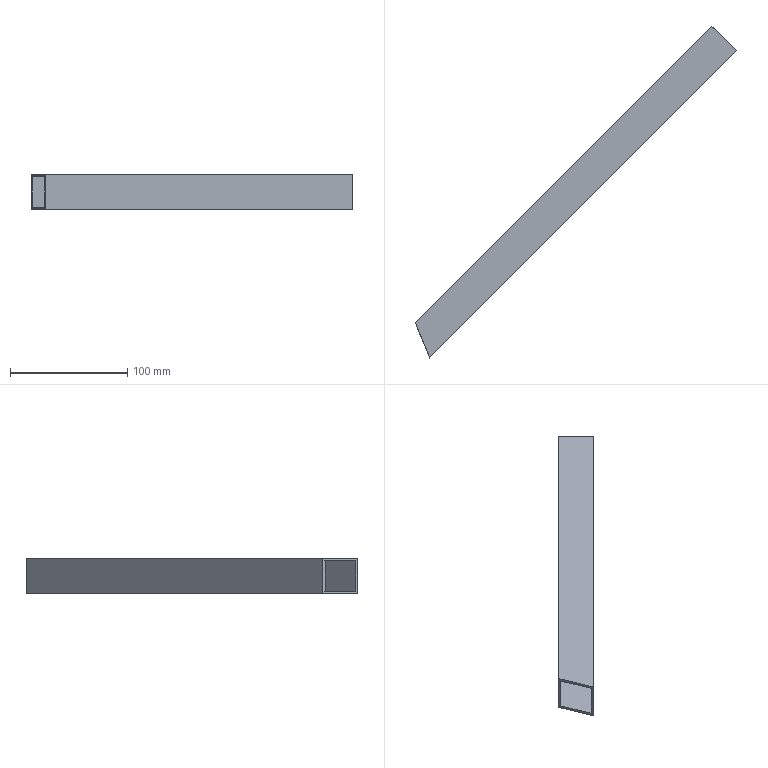Part | NX | features solid 2 | 1 solid | 10 faces | box 274.056 x 282.843 x 30 mm | volume 81488 mm3 | plane 10
STEP:
#1=CARTESIAN_POINT('',(696.63,501.63,-140.));
#2=VERTEX_POINT('',#1);
#3=CARTESIAN_POINT('',(675.416,522.843,-140.));
#4=VERTEX_POINT('',#3);
#5=CARTESIAN_POINT('',(696.63,501.63,-140.));
#6=DIRECTION('',(-0.7071,0.7071,0.));
#7=VECTOR('',#6,1000.);
#8=LINE('',#5,#7);
#9=EDGE_CURVE('',#2,#4,#8,.T.);
#10=ORIENTED_EDGE('',*,*,#9,.T.);
#11=CARTESIAN_POINT('',(675.416,522.843,-110.));
#12=VERTEX_POINT('',#11);
#13=CARTESIAN_POINT('',(675.416,522.843,-110.));
#14=DIRECTION('',(0.,0.,-1.));
#15=VECTOR('',#14,1000.);
#16=LINE('',#13,#15);
#17=EDGE_CURVE('',#12,#4,#16,.T.);
#18=ORIENTED_EDGE('',*,*,#17,.F.);
#19=CARTESIAN_POINT('',(696.63,501.63,-110.));
#20=VERTEX_POINT('',#19);
#21=CARTESIAN_POINT('',(696.63,501.63,-110.));
#22=DIRECTION('',(-0.7071,0.7071,0.));
#23=VECTOR('',#22,1000.);
#24=LINE('',#21,#23);
#25=EDGE_CURVE('',#20,#12,#24,.T.);
#26=ORIENTED_EDGE('',*,*,#25,.F.);
#27=CARTESIAN_POINT('',(696.63,501.63,-110.));
#28=DIRECTION('',(0.,0.,-1.));
#29=VECTOR('',#28,1000.);
#30=LINE('',#27,#29);
#31=EDGE_CURVE('',#20,#2,#30,.T.);
#32=ORIENTED_EDGE('',*,*,#31,.T.);
#33=EDGE_LOOP('',(#10,#18,#26,#32));
#34=FACE_BOUND('',#33,.T.);
#35=CARTESIAN_POINT('',(695.215,503.044,-112.));
#36=VERTEX_POINT('',#35);
#37=CARTESIAN_POINT('',(695.215,503.044,-138.));
#38=VERTEX_POINT('',#37);
#39=CARTESIAN_POINT('',(695.215,503.044,-110.));
#40=DIRECTION('',(0.,0.,-1.));
#41=VECTOR('',#40,1000.);
#42=LINE('',#39,#41);
#43=EDGE_CURVE('',#36,#38,#42,.T.);
#44=ORIENTED_EDGE('',*,*,#43,.F.);
#45=CARTESIAN_POINT('',(676.831,521.428,-112.));
#46=VERTEX_POINT('',#45);
#47=CARTESIAN_POINT('',(696.63,501.63,-112.));
#48=DIRECTION('',(-0.7071,0.7071,0.));
#49=VECTOR('',#48,1000.);
#50=LINE('',#47,#49);
#51=EDGE_CURVE('',#36,#46,#50,.T.);
#52=ORIENTED_EDGE('',*,*,#51,.T.);
#53=CARTESIAN_POINT('',(676.831,521.428,-138.));
#54=VERTEX_POINT('',#53);
#55=CARTESIAN_POINT('',(676.831,521.428,-110.));
#56=DIRECTION('',(0.,0.,-1.));
#57=VECTOR('',#56,1000.);
#58=LINE('',#55,#57);
#59=EDGE_CURVE('',#46,#54,#58,.T.);
#60=ORIENTED_EDGE('',*,*,#59,.T.);
#61=CARTESIAN_POINT('',(696.63,501.63,-138.));
#62=DIRECTION('',(-0.7071,0.7071,0.));
#63=VECTOR('',#62,1000.);
#64=LINE('',#61,#63);
#65=EDGE_CURVE('',#38,#54,#64,.T.);
#66=ORIENTED_EDGE('',*,*,#65,.F.);
#67=EDGE_LOOP('',(#44,#52,#60,#66));
#68=FACE_BOUND('',#67,.T.);
#69=CARTESIAN_POINT('',(696.63,501.63,-110.));
#70=DIRECTION('',(0.7071,0.7071,0.));
#71=DIRECTION('',(0.7071,-0.7071,0.));
#72=AXIS2_PLACEMENT_3D('',#69,#70,#71);
#73=PLANE('',#72);
#74=ADVANCED_FACE('',(#34,#68),#73,.T.);
#75=CARTESIAN_POINT('',(435.,240.,-140.));
#76=VERTEX_POINT('',#75);
#77=CARTESIAN_POINT('',(435.,240.,-140.));
#78=DIRECTION('',(0.7071,0.7071,0.));
#79=VECTOR('',#78,1000.);
#80=LINE('',#77,#79);
#81=EDGE_CURVE('',#76,#2,#80,.T.);
#82=ORIENTED_EDGE('',*,*,#81,.T.);
#83=ORIENTED_EDGE('',*,*,#31,.F.);
#84=CARTESIAN_POINT('',(435.,240.,-110.));
#85=VERTEX_POINT('',#84);
#86=CARTESIAN_POINT('',(435.,240.,-110.));
#87=DIRECTION('',(0.7071,0.7071,0.));
#88=VECTOR('',#87,1000.);
#89=LINE('',#86,#88);
#90=EDGE_CURVE('',#85,#20,#89,.T.);
#91=ORIENTED_EDGE('',*,*,#90,.F.);
#92=CARTESIAN_POINT('',(435.,240.,-110.));
#93=DIRECTION('',(0.,0.,-1.));
#94=VECTOR('',#93,1000.);
#95=LINE('',#92,#94);
#96=EDGE_CURVE('',#85,#76,#95,.T.);
#97=ORIENTED_EDGE('',*,*,#96,.T.);
#98=EDGE_LOOP('',(#82,#83,#91,#97));
#99=FACE_BOUND('',#98,.T.);
#100=CARTESIAN_POINT('',(435.,240.,-110.));
#101=DIRECTION('',(0.7071,-0.7071,0.));
#102=DIRECTION('',(-0.7071,-0.7071,0.));
#103=AXIS2_PLACEMENT_3D('',#100,#101,#102);
#104=PLANE('',#103);
#105=ADVANCED_FACE('',(#99),#104,.T.);
#106=CARTESIAN_POINT('',(422.574,270.,-110.));
#107=VERTEX_POINT('',#106);
#108=CARTESIAN_POINT('',(392.574,240.,-110.));
#109=DIRECTION('',(0.7071,0.7071,0.));
#110=VECTOR('',#109,1000.);
#111=LINE('',#108,#110);
#112=EDGE_CURVE('',#107,#12,#111,.T.);
#113=ORIENTED_EDGE('',*,*,#112,.T.);
#114=ORIENTED_EDGE('',*,*,#17,.T.);
#115=CARTESIAN_POINT('',(422.574,270.,-140.));
#116=VERTEX_POINT('',#115);
#117=CARTESIAN_POINT('',(392.574,240.,-140.));
#118=DIRECTION('',(0.7071,0.7071,0.));
#119=VECTOR('',#118,1000.);
#120=LINE('',#117,#119);
#121=EDGE_CURVE('',#116,#4,#120,.T.);
#122=ORIENTED_EDGE('',*,*,#121,.F.);
#123=CARTESIAN_POINT('',(422.574,270.,-110.));
#124=DIRECTION('',(0.,0.,-1.));
#125=VECTOR('',#124,1000.);
#126=LINE('',#123,#125);
#127=EDGE_CURVE('',#107,#116,#126,.T.);
#128=ORIENTED_EDGE('',*,*,#127,.F.);
#129=EDGE_LOOP('',(#113,#114,#122,#128));
#130=FACE_BOUND('',#129,.T.);
#131=CARTESIAN_POINT('',(392.574,240.,-110.));
#132=DIRECTION('',(0.7071,-0.7071,0.));
#133=DIRECTION('',(-0.7071,-0.7071,0.));
#134=AXIS2_PLACEMENT_3D('',#131,#132,#133);
#135=PLANE('',#134);
#136=ADVANCED_FACE('',(#130),#135,.F.);
#137=CARTESIAN_POINT('',(419.9,276.454,-110.));
#138=DIRECTION('',(0.3827,-0.9239,0.));
#139=VECTOR('',#138,1000.);
#140=LINE('',#137,#139);
#141=EDGE_CURVE('',#107,#85,#140,.T.);
#142=ORIENTED_EDGE('',*,*,#141,.T.);
#143=ORIENTED_EDGE('',*,*,#90,.T.);
#144=ORIENTED_EDGE('',*,*,#25,.T.);
#145=ORIENTED_EDGE('',*,*,#112,.F.);
#146=EDGE_LOOP('',(#142,#143,#144,#145));
#147=FACE_BOUND('',#146,.T.);
#148=CARTESIAN_POINT('',(489.801,305.407,-110.));
#149=DIRECTION('',(0.,0.,1.));
#150=DIRECTION('',(-1.,0.,0.));
#151=AXIS2_PLACEMENT_3D('',#148,#149,#150);
#152=PLANE('',#151);
#153=ADVANCED_FACE('',(#147),#152,.T.);
#154=ORIENTED_EDGE('',*,*,#121,.T.);
#155=ORIENTED_EDGE('',*,*,#9,.F.);
#156=ORIENTED_EDGE('',*,*,#81,.F.);
#157=CARTESIAN_POINT('',(419.9,276.454,-140.));
#158=DIRECTION('',(0.3827,-0.9239,0.));
#159=VECTOR('',#158,1000.);
#160=LINE('',#157,#159);
#161=EDGE_CURVE('',#116,#76,#160,.T.);
#162=ORIENTED_EDGE('',*,*,#161,.F.);
#163=EDGE_LOOP('',(#154,#155,#156,#162));
#164=FACE_BOUND('',#163,.T.);
#165=CARTESIAN_POINT('',(489.801,305.407,-140.));
#166=DIRECTION('',(0.,0.,1.));
#167=DIRECTION('',(-1.,0.,0.));
#168=AXIS2_PLACEMENT_3D('',#165,#166,#167);
#169=PLANE('',#168);
#170=ADVANCED_FACE('',(#164),#169,.F.);
#171=CARTESIAN_POINT('',(423.402,268.,-112.));
#172=VERTEX_POINT('',#171);
#173=CARTESIAN_POINT('',(434.172,242.,-112.));
#174=VERTEX_POINT('',#173);
#175=CARTESIAN_POINT('',(419.9,276.454,-112.));
#176=DIRECTION('',(0.3827,-0.9239,0.));
#177=VECTOR('',#176,1000.);
#178=LINE('',#175,#177);
#179=EDGE_CURVE('',#172,#174,#178,.T.);
#180=ORIENTED_EDGE('',*,*,#179,.T.);
#181=CARTESIAN_POINT('',(434.172,242.,-138.));
#182=VERTEX_POINT('',#181);
#183=CARTESIAN_POINT('',(434.172,242.,-110.));
#184=DIRECTION('',(0.,0.,-1.));
#185=VECTOR('',#184,1000.);
#186=LINE('',#183,#185);
#187=EDGE_CURVE('',#174,#182,#186,.T.);
#188=ORIENTED_EDGE('',*,*,#187,.T.);
#189=CARTESIAN_POINT('',(423.402,268.,-138.));
#190=VERTEX_POINT('',#189);
#191=CARTESIAN_POINT('',(419.9,276.454,-138.));
#192=DIRECTION('',(0.3827,-0.9239,0.));
#193=VECTOR('',#192,1000.);
#194=LINE('',#191,#193);
#195=EDGE_CURVE('',#190,#182,#194,.T.);
#196=ORIENTED_EDGE('',*,*,#195,.F.);
#197=CARTESIAN_POINT('',(423.402,268.,-110.));
#198=DIRECTION('',(0.,0.,-1.));
#199=VECTOR('',#198,1000.);
#200=LINE('',#197,#199);
#201=EDGE_CURVE('',#172,#190,#200,.T.);
#202=ORIENTED_EDGE('',*,*,#201,.F.);
#203=EDGE_LOOP('',(#180,#188,#196,#202));
#204=FACE_BOUND('',#203,.T.);
#205=ORIENTED_EDGE('',*,*,#127,.T.);
#206=ORIENTED_EDGE('',*,*,#161,.T.);
#207=ORIENTED_EDGE('',*,*,#96,.F.);
#208=ORIENTED_EDGE('',*,*,#141,.F.);
#209=EDGE_LOOP('',(#205,#206,#207,#208));
#210=FACE_BOUND('',#209,.T.);
#211=CARTESIAN_POINT('',(435.,240.,-110.));
#212=DIRECTION('',(0.9239,0.3827,0.));
#213=DIRECTION('',(0.3827,-0.9239,0.));
#214=AXIS2_PLACEMENT_3D('',#211,#212,#213);
#215=PLANE('',#214);
#216=ADVANCED_FACE('',(#204,#210),#215,.F.);
#217=CARTESIAN_POINT('',(433.586,241.414,-138.));
#218=DIRECTION('',(0.7071,0.7071,0.));
#219=VECTOR('',#218,1000.);
#220=LINE('',#217,#219);
#221=EDGE_CURVE('',#182,#38,#220,.T.);
#222=ORIENTED_EDGE('',*,*,#221,.F.);
#223=ORIENTED_EDGE('',*,*,#187,.F.);
#224=CARTESIAN_POINT('',(433.586,241.414,-112.));
#225=DIRECTION('',(0.7071,0.7071,0.));
#226=VECTOR('',#225,1000.);
#227=LINE('',#224,#226);
#228=EDGE_CURVE('',#174,#36,#227,.T.);
#229=ORIENTED_EDGE('',*,*,#228,.T.);
#230=ORIENTED_EDGE('',*,*,#43,.T.);
#231=EDGE_LOOP('',(#222,#223,#229,#230));
#232=FACE_BOUND('',#231,.T.);
#233=CARTESIAN_POINT('',(433.586,241.414,-110.));
#234=DIRECTION('',(0.7071,-0.7071,0.));
#235=DIRECTION('',(-0.7071,-0.7071,0.));
#236=AXIS2_PLACEMENT_3D('',#233,#234,#235);
#237=PLANE('',#236);
#238=ADVANCED_FACE('',(#232),#237,.F.);
#239=CARTESIAN_POINT('',(393.988,238.586,-112.));
#240=DIRECTION('',(0.7071,0.7071,0.));
#241=VECTOR('',#240,1000.);
#242=LINE('',#239,#241);
#243=EDGE_CURVE('',#172,#46,#242,.T.);
#244=ORIENTED_EDGE('',*,*,#243,.F.);
#245=ORIENTED_EDGE('',*,*,#201,.T.);
#246=CARTESIAN_POINT('',(393.988,238.586,-138.));
#247=DIRECTION('',(0.7071,0.7071,0.));
#248=VECTOR('',#247,1000.);
#249=LINE('',#246,#248);
#250=EDGE_CURVE('',#190,#54,#249,.T.);
#251=ORIENTED_EDGE('',*,*,#250,.T.);
#252=ORIENTED_EDGE('',*,*,#59,.F.);
#253=EDGE_LOOP('',(#244,#245,#251,#252));
#254=FACE_BOUND('',#253,.T.);
#255=CARTESIAN_POINT('',(393.988,238.586,-110.));
#256=DIRECTION('',(0.7071,-0.7071,0.));
#257=DIRECTION('',(-0.7071,-0.7071,0.));
#258=AXIS2_PLACEMENT_3D('',#255,#256,#257);
#259=PLANE('',#258);
#260=ADVANCED_FACE('',(#254),#259,.T.);
#261=ORIENTED_EDGE('',*,*,#179,.F.);
#262=ORIENTED_EDGE('',*,*,#243,.T.);
#263=ORIENTED_EDGE('',*,*,#51,.F.);
#264=ORIENTED_EDGE('',*,*,#228,.F.);
#265=EDGE_LOOP('',(#261,#262,#263,#264));
#266=FACE_BOUND('',#265,.T.);
#267=CARTESIAN_POINT('',(489.801,305.407,-112.));
#268=DIRECTION('',(0.,0.,1.));
#269=DIRECTION('',(-1.,0.,0.));
#270=AXIS2_PLACEMENT_3D('',#267,#268,#269);
#271=PLANE('',#270);
#272=ADVANCED_FACE('',(#266),#271,.F.);
#273=ORIENTED_EDGE('',*,*,#250,.F.);
#274=ORIENTED_EDGE('',*,*,#195,.T.);
#275=ORIENTED_EDGE('',*,*,#221,.T.);
#276=ORIENTED_EDGE('',*,*,#65,.T.);
#277=EDGE_LOOP('',(#273,#274,#275,#276));
#278=FACE_BOUND('',#277,.T.);
#279=CARTESIAN_POINT('',(489.801,305.407,-138.));
#280=DIRECTION('',(0.,0.,1.));
#281=DIRECTION('',(-1.,0.,0.));
#282=AXIS2_PLACEMENT_3D('',#279,#280,#281);
#283=PLANE('',#282);
#284=ADVANCED_FACE('',(#278),#283,.T.);
#285=CLOSED_SHELL('',(#74,#105,#136,#153,#170,#216,#238,#260,#272,#284));
#286=MANIFOLD_SOLID_BREP('',#285);
#287=(LENGTH_UNIT()NAMED_UNIT(*)SI_UNIT(.MILLI.,.METRE.));
#288=UNCERTAINTY_MEASURE_WITH_UNIT(LENGTH_MEASURE(0.00001),#287,'','');
#289=(NAMED_UNIT(*)PLANE_ANGLE_UNIT()SI_UNIT($,.RADIAN.));
#290=(NAMED_UNIT(*)SI_UNIT($,.STERADIAN.)SOLID_ANGLE_UNIT());
#291=(GEOMETRIC_REPRESENTATION_CONTEXT(3)GLOBAL_UNCERTAINTY_ASSIGNED_CONTEXT((#288))GLOBAL_UNIT_ASSIGNED_CONTEXT((#287,#289,#290))REPRESENTATION_CONTEXT('',''));
#292=ADVANCED_BREP_SHAPE_REPRESENTATION('',(#286),#291);